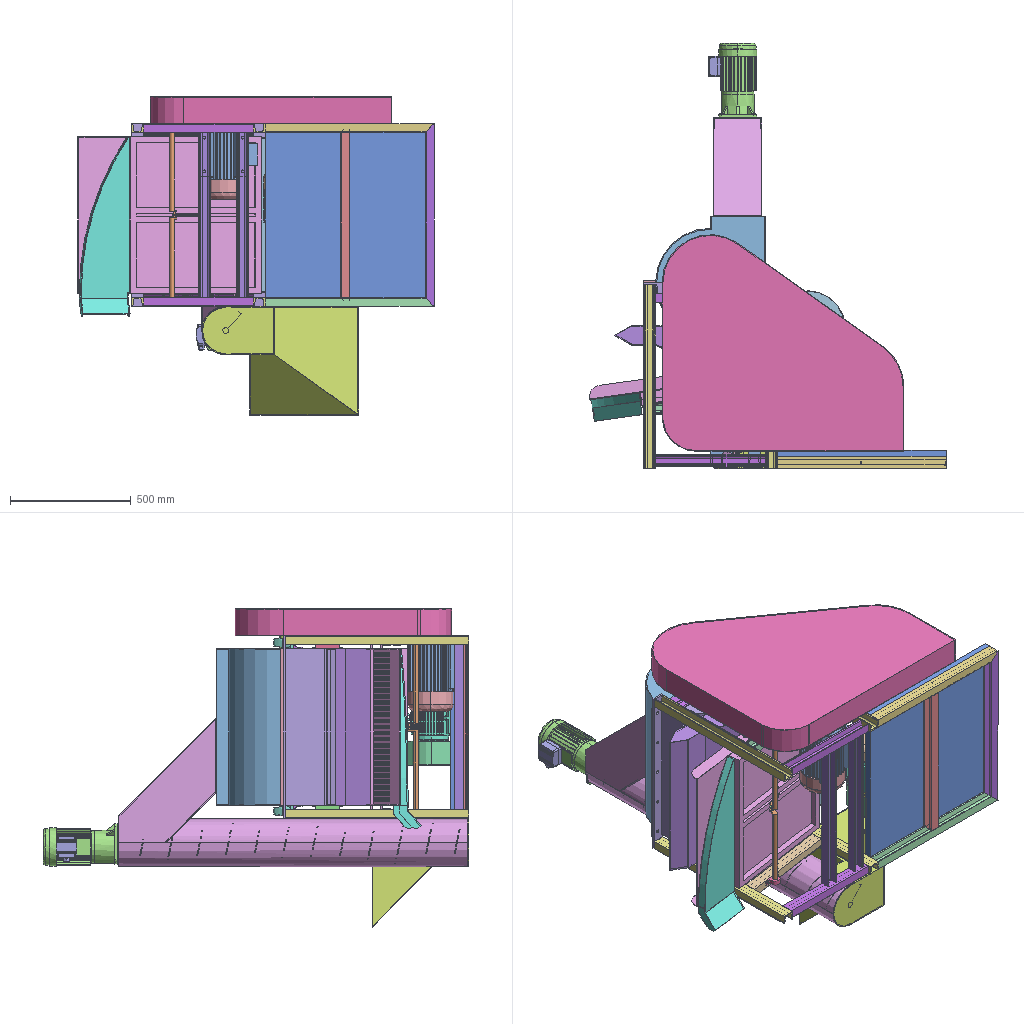Assembly | SolidWorks | 55 different items | 81 placed | box 1477 x 1763 x 1318 mm
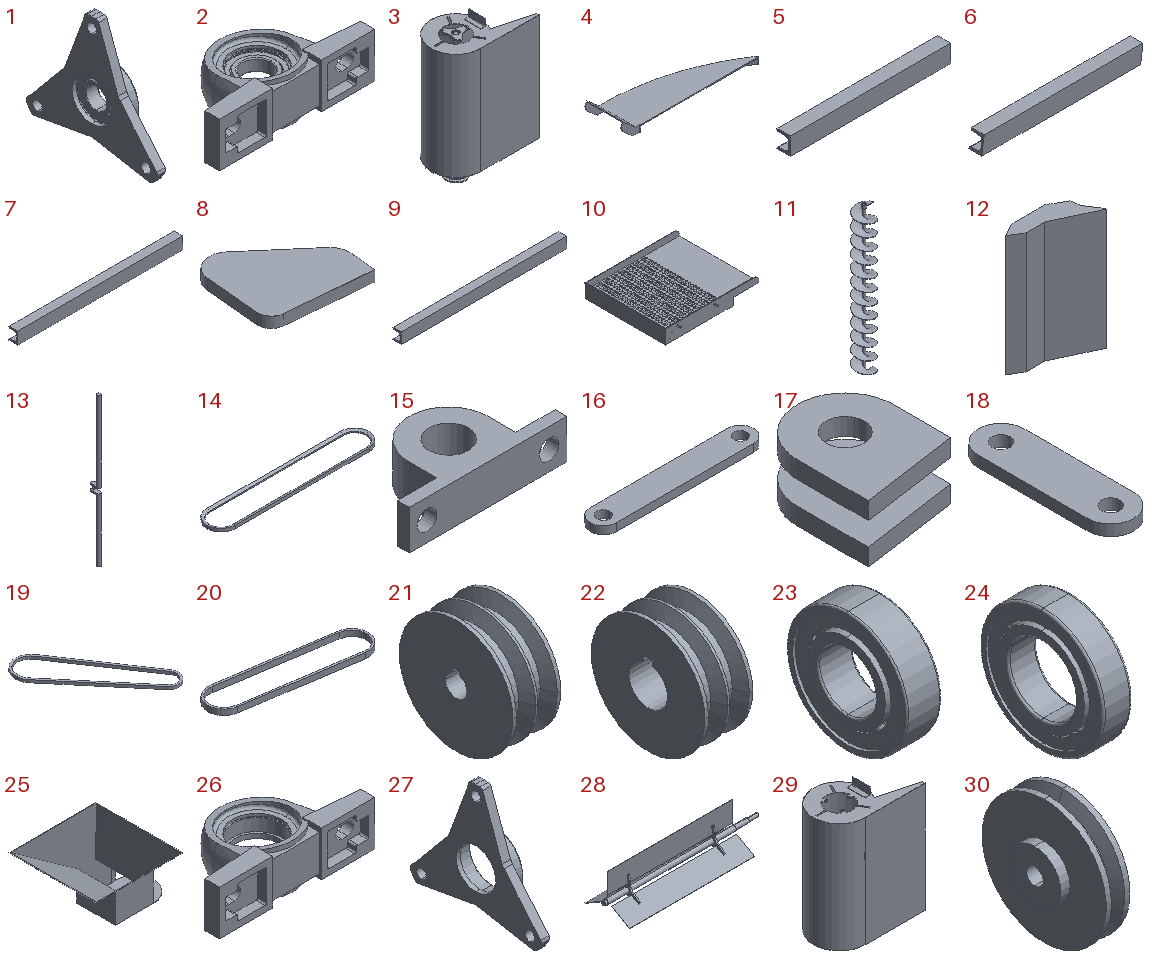Parts list (item | name | quantity | parent item | size | volume | features):
1 | (subassembly) | x2 | in 3 | 16 x 125.605 x 109.685 mm | 58698 mm3 | -
2 | (subassembly) | x2 | - | 167 x 85.5 x 48 mm | 200278 mm3 | -
3 | (subassembly) | x1 | - | 500 x 300 x 787 mm | 3135900 mm3 | -
4 | - | x1 | - | 744.916 x 205 x 90.512 mm | 566343 mm3 | features Shell 2, Extrusion 1, Fillet 1, ICE 1
5 | - | x4 | - | 454 x 37 x 50 mm | 314305 mm3 | features WeldMemberFeat 1, WeldmentFeature 1
6 | - | x1 | - | 465.489 x 37 x 50 mm | 317394 mm3 | features ICE 1, WeldMemberFeat 1, WeldmentFeature 1
7 | - | x2 | - | 684 x 37 x 50 mm | 473534 mm3 | features WeldMemberFeat 1, WeldmentFeature 1
8 | - | x1 | - | 1010 x 967.019 x 110 mm | 3119337 mm3 | features Extrusion 1, Shell 1
9 | - | x4 | - | 760 x 37 x 50 mm | 526149 mm3 | features WeldMemberFeat 1, WeldmentFeature 1
10 | - | x1 | - | 760 x 700 x 113 mm | 5573180 mm3 | features ICE 11, LPattern 2, Extrusion 1, Fillet 1
11 | - | x1 | - | 190 x 190 x 1450 mm | 2067937 mm3 | features ICE 2, Chamfer 1, Extrusion 1, Helix 1, Sweep 1
12 | - | x1 | - | 397.808 x 185.717 x 650 mm | 1840134 mm3 | features ICE 3, Extrusion 1, Shell 1
13 | - | x1 | - | 20 x 50 x 819.2 mm | 260469 mm3 | features ICE 5, Extrusion 1
14 | - | x1 | - | 680.1 x 120.1 x 13 mm | 151786 mm3 | features Sweep 1
15 | - | x2 | - | 80 x 40 x 20 mm | 26141 mm3 | features Extrusion 1, ICE 1
16 | - | x1 | - | 125 x 20 x 6 mm | 13542 mm3 | features Extrusion 1
17 | - | x4 | - | 25 x 31.014 x 15 mm | 5272 mm3 | features Extrusion 1, ICE 1
18 | - | x4 | - | 25 x 85 x 6 mm | 11003 mm3 | features Extrusion 1
19 | - | x3 | - | 410 x 503.461 x 13 mm | 170318 mm3 | features BeltProfileFeature 1, ExtruThin 1
20 | - | x2 | - | 440 x 152.5 x 17 mm | 100304 mm3 | features BeltProfileFeature 1, ExtruThin 1
21 | - | x1 | - | 54 x 100 x 100 mm | 266067 mm3 | features ICE 2, Chamfer 1, HoleWzd 1, Revolution 1
22 | - | x1 | - | 54 x 100 x 100 mm | 231745 mm3 | features ICE 2, Chamfer 1, HoleWzd 1, Revolution 1
23 | - | x2 | in 1 | 12 x 42 x 42 mm | 7887 mm3 | features BaseBody 1
24 | - | x2 | in 2 | 13 x 55 x 55 mm | 14069 mm3 | features BaseBody 1
25 | - | x1 | - | 650 x 450 x 400 mm | 1573727 mm3 | features ICE 2, Blend 1, Extrusion 1, Shell 1
26 | - | x2 | in 2 | 167 x 85.5 x 48 mm | 186208 mm3 | features BaseBody 1
27 | - | x2 | in 1 | 16 x 125.605 x 109.685 mm | 50811 mm3 | features BaseBody 1
28 | - | x1 | in 3 | 751 x 217.506 x 188.366 mm | 750976 mm3 | features BaseBody 6, ICE 3
29 | - | x1 | in 3 | 500 x 300 x 720 mm | 2031659 mm3 | features ICE 4, BaseBody 3
30 | - | x1 | in 3 | 32 x 120 x 120 mm | 235868 mm3 | features BaseBody 1
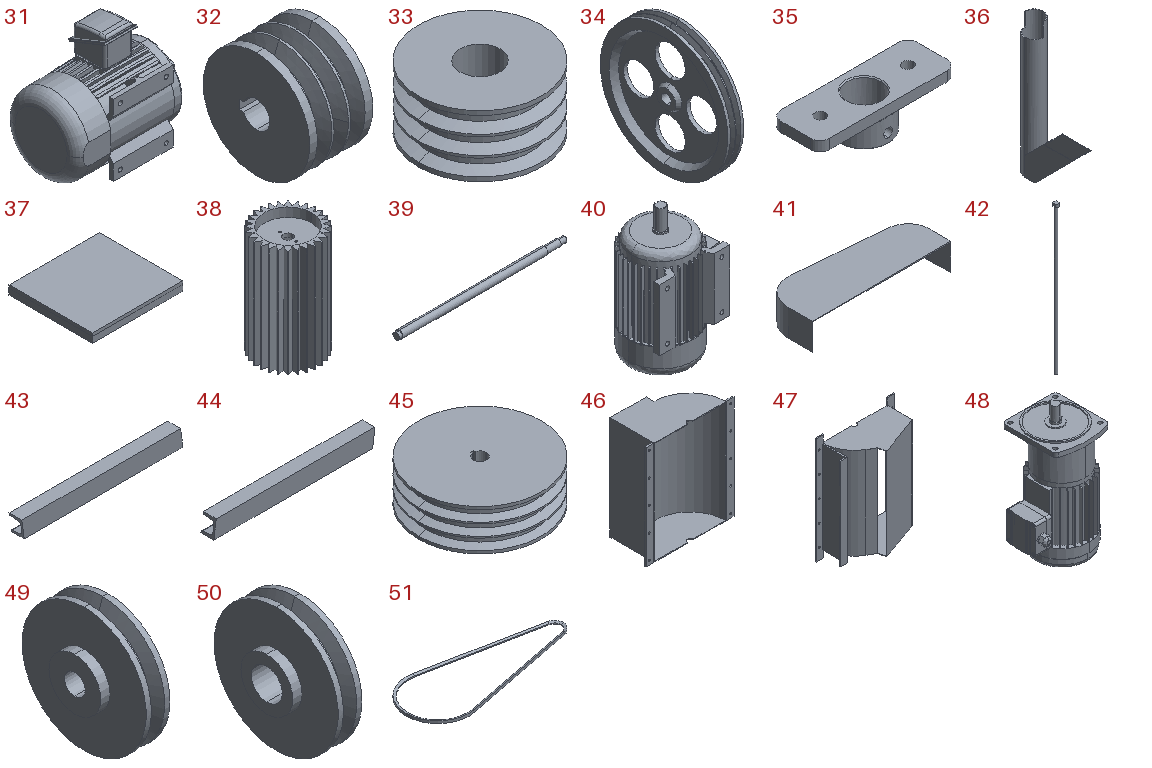31 | - | x1 | - | 282.5 x 193.757 x 234.166 mm | 4079530 mm3 | features ICE 14, Fillet 10, CirPattern 2, Revolution 2, MirrorPattern 1, Shell 1, Sweep 1
32 | - | x1 | - | 66 x 96 x 96 mm | 312790 mm3 | features BaseBody 1
33 | - | x1 | - | 100 x 100 x 50 mm | 274116 mm3 | features ICE 6, Extrusion 1, RevCut 1
34 | - | x1 | - | 42 x 336 x 336 mm | 1380304 mm3 | features BaseBody 1
35 | - | x2 | - | 140 x 50 x 35 mm | 81620 mm3 | features BaseBody 1
36 | - | x1 | - | 200 x 616.127 x 1450 mm | 4635589 mm3 | features ICE 5, Shell 2, Extrusion 1
37 | - | x1 | - | 758 x 700 x 75 mm | 15208825 mm3 | features ICE 1, WeldMemberFeat 1, WeldmentFeature 1
38 | - | x1 | - | 338.194 x 338.194 x 590 mm | 24931977 mm3 | features BaseBody 1, ICE 1
39 | - | x1 | - | 796 x 35 x 35 mm | 731284 mm3 | features BaseBody 1
40 | - | x1 | - | 242.5 x 196 x 380 mm | 6368698 mm3 | features BaseBody 2
41 | - | x1 | - | 520 x 190 x 100 mm | 493401 mm3 | features FlatPattern 1, SMBaseFlange 1, SheetMetal 1, Shell 1
42 | - | x2 | - | 12 x 16 x 545 mm | 43739 mm3 | features BaseBody 1
43 | - | x1 | - | 465.489 x 37 x 50 mm | 317394 mm3 | features MirrorStock 1
44 | - | x1 | - | 465.489 x 37 x 50 mm | 317394 mm3 | features MirrorStock 1
45 | - | x1 | - | 150 x 150 x 50 mm | 752119 mm3 | features ICE 5, Extrusion 1, HoleWzd 1, RevCut 1
46 | - | x1 | - | 554 x 277 x 650 mm | 3183644 mm3 | features ICE 5, LPattern 2, Extrusion 1
47 | - | x1 | - | 554 x 280.82 x 758 mm | 5312644 mm3 | features ICE 8, LPattern 2, Extrusion 1
48 | - | x1 | - | 201.05 x 175.7 x 355 mm | 5359674 mm3 | features BaseBody 2
49 | - | x1 | - | 32 x 120 x 120 mm | 232249 mm3 | features BaseBody 1, ICE 1
50 | - | x1 | - | 32 x 120 x 120 mm | 219683 mm3 | features BaseBody 1, ICE 1
51 | - | x2 | - | 835.6 x 335.6 x 13 mm | 197670 mm3 | features Sweep 1
52 | Two-stage reducerAssembly (subassembly) | x1 | - | - | - | -
53 | Reducer | x1 | - | - | - | -
54 | Drum screen | x1 | - | - | - | -
55 | Assembly1 (subassembly) | x1 | - | - | - | -
Mates (type | each side: item.copy, entity, surface, feature):
In the top assembly
Concentric | 38.1 face cylinder Input 1 | 39.1 face cylinder Input 1
Concentric | 39.1 face cylinder Input 1 | 35.1 face cylinder Input 1
Concentric | 35.2 face cylinder Input 1 | 39.1 face cylinder Input 1
Concentric | 35.2 face cylinder Input 1 | 42.1 face cylinder Input 1
Concentric | 35.2 face cylinder Input 1 | 42.2 face cylinder Input 1
Coincident | 35.2 face plane Input 1 | 42.1 face plane Input 1
Coincident | 35.2 face plane Input 1 | 42.2 face plane Input 1
Concentric | 35.1 face cylinder Input 1 | 42.2 face cylinder Input 1
Coincident | 35.1 face plane Input 1 | 42.2 face plane Input 1
Width | 35.2 face plane Input 1 | 35.1 face plane Input 1 | 38.1 face plane Input 1 | 38.1 face plane Input 1
Coincident | 38.1 face cylinder Cut-Extrude1 | 42.1 edge
Concentric | 39.1 face cylinder Input 1 | 24.1 face cylinder Input 1
Concentric | 39.1 face cylinder Input 1 | 24.2 face cylinder Input 1
Coincident | 39.1 face plane Input 1 | 24.1 face plane Input 1
Coincident | 39.1 face plane Input 1 | 24.2 face plane Input 1
Width | 26.1 face plane Input 1 | 26.2 face plane Input 1 | 38.1 face plane Input 1 | 38.1 face plane Input 1
Parallel | 35.2 edge | 26.1 face plane Input 1
Coincident | 26.2 face plane Input 1 | 26.1 face plane Input 1
Width | 29.1 face plane Input 1 | 29.1 face plane Input 1 | 47.1 face plane Boss-Extrude2 | 47.1 face plane Boss-Extrude2
Parallel | 26.1 face plane Input 1 | 47.1 face plane Boss-Extrude2
Coincident | 47.1 face plane Cut-Extrude3 | 12.1 face plane Boss-Extrude1
Width | 12.1 face plane Boss-Extrude1 | 12.1 face plane Boss-Extrude1 | 47.1 face plane Boss-Extrude2 | 47.1 face plane Boss-Extrude2
Coincident | 47.1 face cylinder Boss-Extrude2 | 12.1 edge
Concentric | 39.1 face cylinder Input 1 | 34.1 face cylinder Input 1
Coincident | 39.1 face plane Input 1 | 34.1 face plane Input 1
Concentric | 40.1 face cylinder Input 2 | 32.1 face cylinder Input 1
Coincident | 40.1 face plane Input 2 | 32.1 face plane Input 1
Coincident | 34.1 face plane Input 1 | 32.1 face plane Input 1
Width | 10.1 face plane Boss-Extrude1 | 10.1 face plane Boss-Extrude1 | 47.1 face plane Boss-Extrude2 | 47.1 face plane Boss-Extrude2
Concentric | 34.1 face cylinder Input 1 | 51.1 face cylinder Sweep1
Coincident | 34.1 edge | 51.1 edge
Concentric | 32.1 face cylinder Input 1 | 51.1 face cylinder Sweep1
Concentric | 34.1 face cylinder Input 1 | 51.2 face cylinder Sweep1
Coincident | 34.1 edge | 51.2 edge
Concentric | 32.1 face cylinder Input 1 | 51.2 face cylinder Sweep1
Concentric | 13.1 face cylinder Boss-Extrude1 | 49.1 face cylinder Cut-Extrude1 | 2 times
Concentric | 13.1 face cylinder Boss-Extrude3 | 16.1 face cylinder Boss-Extrude1
Width | 16.1 face plane Boss-Extrude1 | 16.1 face plane Boss-Extrude1 | 13.1 face plane Boss-Extrude2 | 13.1 face plane Boss-Extrude2
Concentric | 13.1 face cylinder Boss-Extrude1 | 15.1 face cylinder Boss-Extrude1
Concentric | 49.1 face cylinder Input 1 | 14.1 face cylinder Sweep1
Concentric | 10.1 face cylinder Cut-Extrude4 | 16.1 face cylinder Boss-Extrude1
Coincident | 47.1 face plane Boss-Extrude2 | 9.1 face plane GB/T 707-1988 hot-rolled channel 05(1) | 2 times
Coincident | 47.1 face plane Boss-Extrude6 | 9.1 face plane GB/T 707-1988 hot-rolled channel 05(1)
Coincident | 47.1 face plane Boss-Extrude2 | 9.2 face plane GB/T 707-1988 hot-rolled channel 05(1) | 2 times
Coincident | 47.1 face plane Boss-Extrude6 | 9.2 face plane GB/T 707-1988 hot-rolled channel 05(1)
Coincident | 26.2 face plane Input 1 | 5.1 face plane GB/T 707-1988 hot-rolled channel 05(1) | 2 times
Coincident | 9.1 face plane GB/T 707-1988 hot-rolled channel 05(1) | 5.1 face plane GB/T 707-1988 hot-rolled channel 05(1)
Coincident | 47.1 face plane Boss-Extrude2 | 9.3 face plane GB/T 707-1988 hot-rolled channel 05(1) | 2 times
Coincident | 47.1 face plane Boss-Extrude6 | 9.3 face plane GB/T 707-1988 hot-rolled channel 05(1)
Coincident | 47.1 face plane Boss-Extrude2 | 9.4 face plane GB/T 707-1988 hot-rolled channel 05(1) | 2 times
Coincident | 47.1 face plane Boss-Extrude6 | 9.4 face plane GB/T 707-1988 hot-rolled channel 05(1)
Coincident | 26.1 face plane Input 1 | 5.2 face plane GB/T 707-1988 hot-rolled channel 05(1) | 2 times
Coincident | 9.3 face plane GB/T 707-1988 hot-rolled channel 05(1) | 5.2 face plane GB/T 707-1988 hot-rolled channel 05(1)
Coincident | 9.3 face plane GB/T 707-1988 hot-rolled channel 05(1) | 43.1 face plane 20260326 Crossbeam454 Inclined_Mirror | 2 times
Concentric | 39.1 edge | 50.1 face cylinder Cut-Extrude1
Coincident | 34.1 face plane Input 1 | 50.1 face plane Input 1
Concentric | 14.1 face cylinder Sweep1 | 50.1 face cylinder Input 1
Coincident | 49.1 face plane Input 1 | 50.1 face plane Input 1
Coincident | 15.1 face plane Boss-Extrude1 | 43.1 face plane 20260326 Crossbeam454 Inclined_Mirror | 2 times
Concentric | 10.1 face cylinder Boss-Extrude4 | 18.1 face cylinder Boss-Extrude1
Coincident | 10.1 face plane Boss-Extrude4 | 18.1 face plane Boss-Extrude1
Concentric | 17.1 face cylinder Boss-Extrude1 | 18.1 face cylinder Boss-Extrude1
Coincident | 43.1 face plane 20260326 Crossbeam454 Inclined_Mirror | 17.1 face plane Boss-Extrude1
Width | 18.1 face plane Boss-Extrude1 | 18.1 face plane Boss-Extrude1 | 17.1 face plane Boss-Extrude1 | 17.1 face plane Boss-Extrude1
Coincident | 18.1 face plane Boss-Extrude1 | 18.2 face plane Boss-Extrude1
Concentric | 10.1 face cylinder Boss-Extrude4 | 18.2 face cylinder Boss-Extrude1
Concentric | 18.2 face cylinder Boss-Extrude1 | 17.2 face cylinder Boss-Extrude1
Coincident | 17.1 face plane Boss-Extrude1 | 17.2 face plane Boss-Extrude1
Coincident | 43.1 edge | 17.2 face plane Boss-Extrude1
DistanceDim | 17.2 face cylinder Boss-Extrude1 | 17.1 face cylinder Boss-Extrude1
Width | 17.1 face plane Boss-Extrude1 | 17.2 face plane Boss-Extrude1 | 9.3 face plane GB/T 707-1988 hot-rolled channel 05(1) | 9.4 face plane GB/T 707-1988 hot-rolled channel 05(1)
DistanceDim | 14.1 edge | 50.1 face plane Input 1
DistanceDim | 15.1 edge | 9.4 face plane GB/T 707-1988 hot-rolled channel 05(1)
Width | 16.1 face plane Boss-Extrude1 | 16.1 face plane Boss-Extrude1 | 10.1 face plane Boss-Extrude10 | 10.1 face plane Boss-Extrude10
Coincident | 10.1 face plane Boss-Extrude1 | 4.1 face plane Boss-Extrude1
Coincident | 10.1 face plane Boss-Extrude8 | 4.1 face plane Boss-Extrude1
Coincident | 44.1 face plane Mirror20260326 Crossbeam454 Inclined_Mirror | 15.2 face plane Boss-Extrude1 | 2 times
Concentric | 13.1 face cylinder Boss-Extrude1 | 15.2 face cylinder Boss-Extrude1
Parallel | 40.1 face plane Input 2 | 9.3 face plane GB/T 707-1988 hot-rolled channel 05(1)
DistanceDim | 40.1 face plane Input 2 | 9.3 face plane GB/T 707-1988 hot-rolled channel 05(1)
Coincident | 29.1 face plane Input 3 | 9.3 face plane GB/T 707-1988 hot-rolled channel 05(1) | 2 times
Coincident | 40.1 face plane Input 2 | 5.3 face plane GB/T 707-1988 hot-rolled channel 05(1)
Coincident | 9.3 face plane GB/T 707-1988 hot-rolled channel 05(1) | 5.3 face plane GB/T 707-1988 hot-rolled channel 05(1) | 2 times
Coincident | 9.2 face plane GB/T 707-1988 hot-rolled channel 05(1) | 5.4 face plane GB/T 707-1988 hot-rolled channel 05(1)
Coincident | 5.3 face plane GB/T 707-1988 hot-rolled channel 05(1) | 5.4 face plane GB/T 707-1988 hot-rolled channel 05(1)
Coincident | 9.1 face plane GB/T 707-1988 hot-rolled channel 05(1) | 5.4 face plane GB/T 707-1988 hot-rolled channel 05(1)
Coincident | 5.4 face plane GB/T 707-1988 hot-rolled channel 05(1) | 7.1 face plane GB/T 707-1988 hot-rolled channel 05(1)
Coincident | 5.3 face plane GB/T 707-1988 hot-rolled channel 05(1) | 7.1 face plane GB/T 707-1988 hot-rolled channel 05(1)
Coincident | 40.1 face plane Input 2 | 7.1 face plane GB/T 707-1988 hot-rolled channel 05(1)
Coincident | 40.1 face plane Input 2 | 7.2 face plane GB/T 707-1988 hot-rolled channel 05(1)
Coincident | 7.1 face plane GB/T 707-1988 hot-rolled channel 05(1) | 7.2 face plane GB/T 707-1988 hot-rolled channel 05(1)
Coincident | 5.4 face plane GB/T 707-1988 hot-rolled channel 05(1) | 7.2 face plane GB/T 707-1988 hot-rolled channel 05(1)
Coincident | 47.1 face plane Boss-Extrude2 | 46.1 face plane Boss-Extrude1 | 2 times
Concentric | 39.1 face cylinder Input 1 | 46.1 face cylinder Cut-Extrude2
Coincident | 9.2 face plane GB/T 707-1988 hot-rolled channel 05(1) | 25.1 face plane Boss-Extrude1 | 2 times
Concentric | 25.1 face cylinder Boss-Extrude2 | 36.1 face cylinder Boss-Extrude1
Coincident | 25.1 face plane Boss-Extrude2 | 36.1 face plane Boss-Extrude1
Coincident | 25.1 edge | 36.1 face plane Cut-Extrude2
Width | 36.1 face plane Boss-Extrude2 | 36.1 face plane Boss-Extrude2 | 46.1 face plane Boss-Extrude1 | 46.1 face plane Boss-Extrude1
Coincident | 25.1 face plane Boss-Extrude2 | 11.1 face plane Boss-Extrude1
Concentric | 36.1 face cylinder Shell5 | 11.1 face cylinder Boss-Extrude1
Concentric | 11.1 face cylinder Cut-Extrude1 | 48.1 face cylinder Input 2
Coincident | 36.1 face plane Boss-Extrude3 | 48.1 face plane Input 2
Parallel | 36.1 edge | 48.1 edge
Width | 46.1 face plane Boss-Extrude1 | 46.1 face plane Boss-Extrude1 | 38.1 face plane Input 1 | 38.1 face plane Input 1
Coincident | 9.4 face plane GB/T 707-1988 hot-rolled channel 05(1) | 8.1 face plane Boss-Extrude2
Concentric | 34.1 face cylinder Input 1 | 8.1 face cylinder Boss-Extrude2
Parallel | 9.4 face plane GB/T 707-1988 hot-rolled channel 05(1) | 8.1 face plane Boss-Extrude2
DistanceDim | 29.1 face plane Input 3 | 47.1 face plane Boss-Extrude2
DistanceDim | 9.3 face plane GB/T 707-1988 hot-rolled channel 05(1) | assembly face
Coincident | 28.1 face plane Boss-Extrude1 | assembly face
Coincident | 28.1 face plane Boss-Extrude1 | 45.1 face plane Boss-Extrude1
Concentric | 28.1 face cylinder Input 2 | 45.1 face cylinder Cut-Extrude1
Coincident | 9.3 face plane GB/T 707-1988 hot-rolled channel 05(1) | 37.1 face plane GB/T 707-1988 hot-rolled channel 5(1) | 3 times
DistanceDim | assembly face | 37.1 face plane GB/T 707-1988 hot-rolled channel 5(1)
Coincident | 37.1 face plane Boss-Extrude1 | assembly face
Coincident | 37.1 face plane Boss-Extrude1 | 31.1 face plane Boss-Extrude1
Coincident | 31.1 face plane Revolve1 | 21.1 face plane Revolve1
Concentric | 31.1 face cylinder Revolve1 | 21.1 face cylinder Cut-Extrude1
Concentric | 45.1 face cylinder Cut-Revolve1 | 19.1 face cylinder Extrude-Thin1
Coincident | 45.1 edge | 19.1 face plane Extrude-Thin1
Coincident | 37.1 face plane Boss-Extrude1 | 41.1 face plane Base-Flange2
Concentric | 33.1 face cylinder Cut-Revolve1 | 19.2 face cylinder Extrude-Thin1
Coincident | 33.1 edge | 19.2 edge
Concentric | 21.1 face cylinder Revolve1 | 20.1 face cylinder Extrude-Thin1
Concentric | 22.1 face cylinder Revolve1 | 20.1 face cylinder Extrude-Thin1
Coincident | 22.1 edge | 20.1 edge
Coincident | 21.1 edge | 20.1 face plane Extrude-Thin1
In subassembly 3
Concentric | 28.2 face cylinder Input 2 | 30.1 face cylinder Input 1
DistanceDim | 30.1 face plane Input 1 | 28.2 face